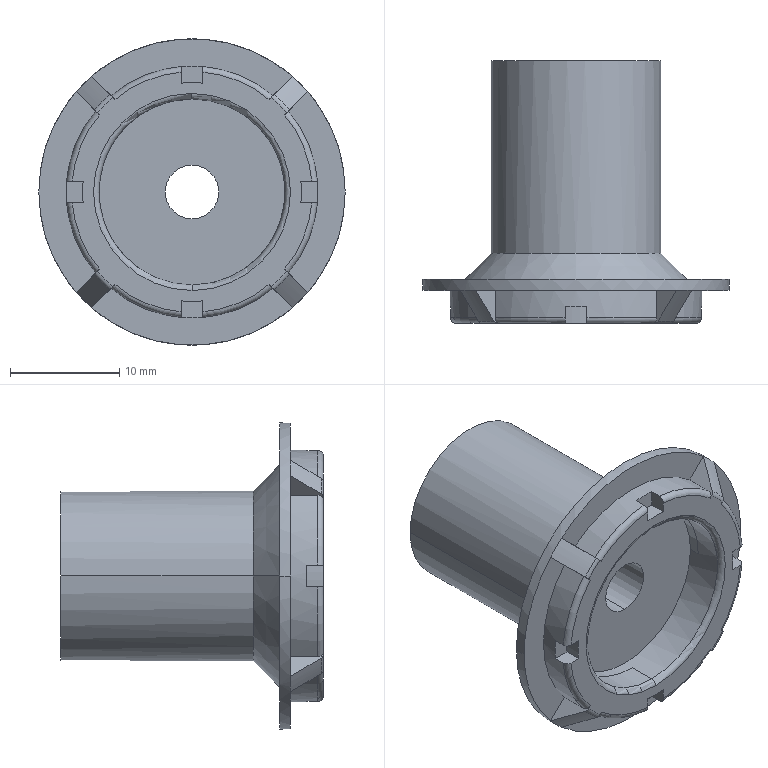Part | STEP file | ZHOUTAO_18_1 | 1 solid | 64 faces | box 28 x 24 x 28 mm | volume 4512 mm3 | plane 28 | cylinder 16 | torus 14 | cone 6 | commonest cylinder face diameters 20 x4 23 x4 4.9 x2 15.5 x2 17 x2 28 x2